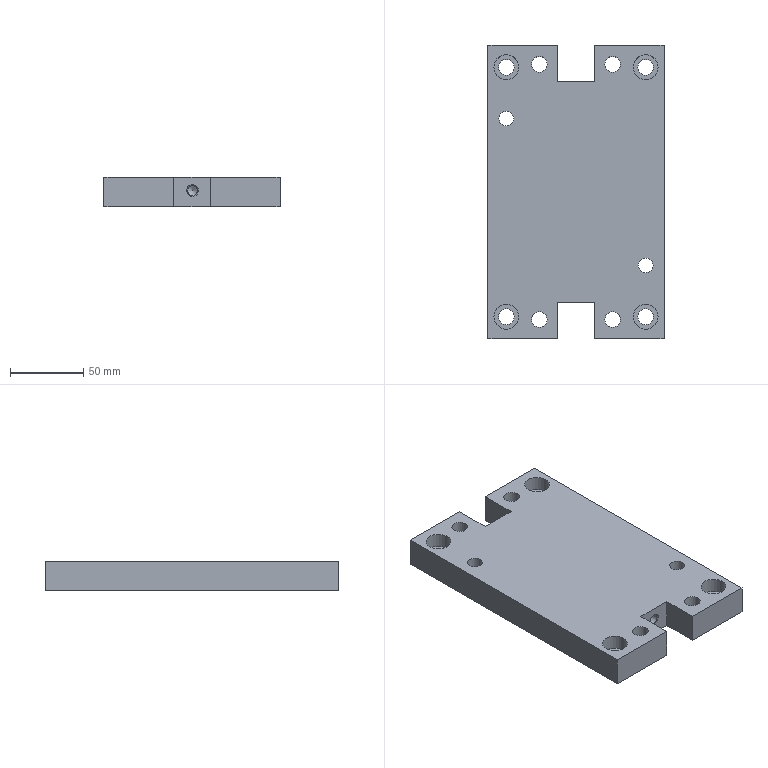Part | STEP file | 冲床-300配套压波_id810_x_t | 1 solid | 46 faces | box 120 x 200 x 20 mm | volume 424966 mm3 | plane 22 | cylinder 20 | cone 4 | commonest cylinder face diameters 10.7 x8 17 x8 6.8 x2 10 x2
STEP:
#1=CARTESIAN_POINT('',(1589.65,87.,10.));
#2=VERTEX_POINT('',#1);
#3=CARTESIAN_POINT('',(1595.,87.,10.));
#4=DIRECTION('',(0.,0.,-1.));
#5=DIRECTION('',(-1.,0.,0.));
#6=AXIS2_PLACEMENT_3D('',#3,#4,#5);
#7=CIRCLE('',#6,5.35);
#8=EDGE_CURVE('',#2,#2,#7,.T.);
#9=ORIENTED_EDGE('',*,*,#8,.F.);
#10=EDGE_LOOP('',(#9));
#11=FACE_BOUND('',#10,.T.);
#12=CARTESIAN_POINT('',(1586.5,87.,10.));
#13=VERTEX_POINT('',#12);
#14=CARTESIAN_POINT('',(1595.,87.,10.));
#15=DIRECTION('',(0.,0.,-1.));
#16=DIRECTION('',(-1.,0.,0.));
#17=AXIS2_PLACEMENT_3D('',#14,#15,#16);
#18=CIRCLE('',#17,8.5);
#19=EDGE_CURVE('',#13,#13,#18,.T.);
#20=ORIENTED_EDGE('',*,*,#19,.T.);
#21=EDGE_LOOP('',(#20));
#22=FACE_BOUND('',#21,.T.);
#23=CARTESIAN_POINT('',(1595.,87.,10.));
#24=DIRECTION('',(0.,0.,1.));
#25=DIRECTION('',(-1.,0.,0.));
#26=AXIS2_PLACEMENT_3D('',#23,#24,#25);
#27=PLANE('',#26);
#28=ADVANCED_FACE('',(#11,#22),#27,.F.);
#29=ORIENTED_EDGE('',*,*,#19,.F.);
#30=EDGE_LOOP('',(#29));
#31=FACE_BOUND('',#30,.T.);
#32=CARTESIAN_POINT('',(1586.5,87.,0.));
#33=VERTEX_POINT('',#32);
#34=CARTESIAN_POINT('',(1595.,87.,0.));
#35=DIRECTION('',(0.,0.,1.));
#36=DIRECTION('',(-1.,0.,0.));
#37=AXIS2_PLACEMENT_3D('',#34,#35,#36);
#38=CIRCLE('',#37,8.5);
#39=EDGE_CURVE('',#33,#33,#38,.T.);
#40=ORIENTED_EDGE('',*,*,#39,.F.);
#41=EDGE_LOOP('',(#40));
#42=FACE_BOUND('',#41,.T.);
#43=CARTESIAN_POINT('',(1595.,87.,0.));
#44=DIRECTION('',(0.,0.,1.));
#45=DIRECTION('',(-1.,0.,0.));
#46=AXIS2_PLACEMENT_3D('',#43,#44,#45);
#47=CYLINDRICAL_SURFACE('',#46,8.5);
#48=ADVANCED_FACE('',(#31,#42),#47,.F.);
#49=CARTESIAN_POINT('',(1589.65,87.,20.));
#50=VERTEX_POINT('',#49);
#51=CARTESIAN_POINT('',(1595.,87.,20.));
#52=DIRECTION('',(0.,0.,-1.));
#53=DIRECTION('',(-1.,0.,0.));
#54=AXIS2_PLACEMENT_3D('',#51,#52,#53);
#55=CIRCLE('',#54,5.35);
#56=EDGE_CURVE('',#50,#50,#55,.T.);
#57=ORIENTED_EDGE('',*,*,#56,.F.);
#58=EDGE_LOOP('',(#57));
#59=FACE_BOUND('',#58,.T.);
#60=ORIENTED_EDGE('',*,*,#8,.T.);
#61=EDGE_LOOP('',(#60));
#62=FACE_BOUND('',#61,.T.);
#63=CARTESIAN_POINT('',(1595.,87.,101.559));
#64=DIRECTION('',(0.,0.,1.));
#65=DIRECTION('',(-1.,0.,0.));
#66=AXIS2_PLACEMENT_3D('',#63,#64,#65);
#67=CYLINDRICAL_SURFACE('',#66,5.35);
#68=ADVANCED_FACE('',(#59,#62),#67,.F.);
#69=CARTESIAN_POINT('',(1623.725,-55.,11.));
#70=VERTEX_POINT('',#69);
#71=CARTESIAN_POINT('',(1620.325,-55.,11.));
#72=DIRECTION('',(0.,-1.,0.));
#73=DIRECTION('',(1.,0.,0.));
#74=AXIS2_PLACEMENT_3D('',#71,#72,#73);
#75=CIRCLE('',#74,3.4);
#76=EDGE_CURVE('',#70,#70,#75,.T.);
#77=ORIENTED_EDGE('',*,*,#76,.T.);
#78=EDGE_LOOP('',(#77));
#79=FACE_BOUND('',#78,.T.);
#80=CARTESIAN_POINT('',(1620.325,-52.957,11.));
#81=VERTEX_POINT('',#80);
#82=VERTEX_LOOP('',#81);
#83=FACE_BOUND('',#82,.T.);
#84=CARTESIAN_POINT('',(1620.325,-55.,11.));
#85=DIRECTION('',(0.,-1.,0.));
#86=DIRECTION('',(-1.,0.,0.));
#87=AXIS2_PLACEMENT_3D('',#84,#85,#86);
#88=CONICAL_SURFACE('',#87,3.4,59.);
#89=ADVANCED_FACE('',(#79,#83),#88,.F.);
#90=CARTESIAN_POINT('',(1623.725,55.,11.));
#91=VERTEX_POINT('',#90);
#92=CARTESIAN_POINT('',(1620.325,55.,11.));
#93=DIRECTION('',(0.,1.,0.));
#94=DIRECTION('',(1.,0.,0.));
#95=AXIS2_PLACEMENT_3D('',#92,#93,#94);
#96=CIRCLE('',#95,3.4);
#97=EDGE_CURVE('',#91,#91,#96,.T.);
#98=ORIENTED_EDGE('',*,*,#97,.T.);
#99=EDGE_LOOP('',(#98));
#100=FACE_BOUND('',#99,.T.);
#101=CARTESIAN_POINT('',(1620.325,52.957,11.));
#102=VERTEX_POINT('',#101);
#103=VERTEX_LOOP('',#102);
#104=FACE_BOUND('',#103,.T.);
#105=CARTESIAN_POINT('',(1620.325,55.,11.));
#106=DIRECTION('',(0.,1.,0.));
#107=DIRECTION('',(-1.,0.,0.));
#108=AXIS2_PLACEMENT_3D('',#105,#106,#107);
#109=CONICAL_SURFACE('',#108,3.4,59.);
#110=ADVANCED_FACE('',(#100,#104),#109,.F.);
#111=CARTESIAN_POINT('',(1620.325,-74.4,14.4));
#112=VERTEX_POINT('',#111);
#113=CARTESIAN_POINT('',(1620.325,-74.4,11.));
#114=DIRECTION('',(0.,-1.,0.));
#115=DIRECTION('',(0.,0.,1.));
#116=AXIS2_PLACEMENT_3D('',#113,#114,#115);
#117=CIRCLE('',#116,3.4);
#118=EDGE_CURVE('',#112,#112,#117,.T.);
#119=ORIENTED_EDGE('',*,*,#118,.T.);
#120=EDGE_LOOP('',(#119));
#121=FACE_BOUND('',#120,.T.);
#122=ORIENTED_EDGE('',*,*,#76,.F.);
#123=EDGE_LOOP('',(#122));
#124=FACE_BOUND('',#123,.T.);
#125=CARTESIAN_POINT('',(1620.325,-75.,11.));
#126=DIRECTION('',(0.,1.,0.));
#127=DIRECTION('',(1.,0.,0.));
#128=AXIS2_PLACEMENT_3D('',#125,#126,#127);
#129=CYLINDRICAL_SURFACE('',#128,3.4);
#130=ADVANCED_FACE('',(#121,#124),#129,.F.);
#131=CARTESIAN_POINT('',(1620.325,74.4,14.4));
#132=VERTEX_POINT('',#131);
#133=CARTESIAN_POINT('',(1620.325,74.4,11.));
#134=DIRECTION('',(0.,1.,0.));
#135=DIRECTION('',(0.,0.,1.));
#136=AXIS2_PLACEMENT_3D('',#133,#134,#135);
#137=CIRCLE('',#136,3.4);
#138=EDGE_CURVE('',#132,#132,#137,.T.);
#139=ORIENTED_EDGE('',*,*,#138,.T.);
#140=EDGE_LOOP('',(#139));
#141=FACE_BOUND('',#140,.T.);
#142=ORIENTED_EDGE('',*,*,#97,.F.);
#143=EDGE_LOOP('',(#142));
#144=FACE_BOUND('',#143,.T.);
#145=CARTESIAN_POINT('',(1620.325,75.,11.));
#146=DIRECTION('',(0.,-1.,0.));
#147=DIRECTION('',(1.,0.,0.));
#148=AXIS2_PLACEMENT_3D('',#145,#146,#147);
#149=CYLINDRICAL_SURFACE('',#148,3.4);
#150=ADVANCED_FACE('',(#141,#144),#149,.F.);
#151=ORIENTED_EDGE('',*,*,#118,.F.);
#152=EDGE_LOOP('',(#151));
#153=FACE_BOUND('',#152,.T.);
#154=CARTESIAN_POINT('',(1616.325,-75.,11.));
#155=VERTEX_POINT('',#154);
#156=CARTESIAN_POINT('',(1620.325,-75.,11.));
#157=DIRECTION('',(0.,1.,0.));
#158=DIRECTION('',(-1.,0.,0.));
#159=AXIS2_PLACEMENT_3D('',#156,#157,#158);
#160=CIRCLE('',#159,4.);
#161=EDGE_CURVE('',#155,#155,#160,.T.);
#162=ORIENTED_EDGE('',*,*,#161,.F.);
#163=EDGE_LOOP('',(#162));
#164=FACE_BOUND('',#163,.T.);
#165=CARTESIAN_POINT('',(1620.325,-75.,11.));
#166=DIRECTION('',(0.,-1.,0.));
#167=DIRECTION('',(0.,0.,1.));
#168=AXIS2_PLACEMENT_3D('',#165,#166,#167);
#169=CONICAL_SURFACE('',#168,4.,45.);
#170=ADVANCED_FACE('',(#153,#164),#169,.F.);
#171=ORIENTED_EDGE('',*,*,#138,.F.);
#172=EDGE_LOOP('',(#171));
#173=FACE_BOUND('',#172,.T.);
#174=CARTESIAN_POINT('',(1616.325,75.,11.));
#175=VERTEX_POINT('',#174);
#176=CARTESIAN_POINT('',(1620.325,75.,11.));
#177=DIRECTION('',(0.,-1.,0.));
#178=DIRECTION('',(-1.,0.,0.));
#179=AXIS2_PLACEMENT_3D('',#176,#177,#178);
#180=CIRCLE('',#179,4.);
#181=EDGE_CURVE('',#175,#175,#180,.T.);
#182=ORIENTED_EDGE('',*,*,#181,.F.);
#183=EDGE_LOOP('',(#182));
#184=FACE_BOUND('',#183,.T.);
#185=CARTESIAN_POINT('',(1620.325,75.,11.));
#186=DIRECTION('',(0.,1.,0.));
#187=DIRECTION('',(0.,0.,1.));
#188=AXIS2_PLACEMENT_3D('',#185,#186,#187);
#189=CONICAL_SURFACE('',#188,4.,45.);
#190=ADVANCED_FACE('',(#173,#184),#189,.F.);
#191=CARTESIAN_POINT('',(1564.,85.,10.));
#192=VERTEX_POINT('',#191);
#193=CARTESIAN_POINT('',(1572.5,85.,10.));
#194=DIRECTION('',(0.,0.,1.));
#195=DIRECTION('',(-1.,0.,0.));
#196=AXIS2_PLACEMENT_3D('',#193,#194,#195);
#197=CIRCLE('',#196,8.5);
#198=EDGE_CURVE('',#192,#192,#197,.T.);
#199=ORIENTED_EDGE('',*,*,#198,.T.);
#200=EDGE_LOOP('',(#199));
#201=FACE_BOUND('',#200,.T.);
#202=CARTESIAN_POINT('',(1567.15,85.,10.));
#203=VERTEX_POINT('',#202);
#204=CARTESIAN_POINT('',(1572.5,85.,10.));
#205=DIRECTION('',(0.,0.,1.));
#206=DIRECTION('',(-1.,0.,0.));
#207=AXIS2_PLACEMENT_3D('',#204,#205,#206);
#208=CIRCLE('',#207,5.35);
#209=EDGE_CURVE('',#203,#203,#208,.T.);
#210=ORIENTED_EDGE('',*,*,#209,.F.);
#211=EDGE_LOOP('',(#210));
#212=FACE_BOUND('',#211,.T.);
#213=CARTESIAN_POINT('',(1572.5,85.,10.));
#214=DIRECTION('',(0.,0.,-1.));
#215=DIRECTION('',(-1.,0.,0.));
#216=AXIS2_PLACEMENT_3D('',#213,#214,#215);
#217=PLANE('',#216);
#218=ADVANCED_FACE('',(#201,#212),#217,.F.);
#219=CARTESIAN_POINT('',(1676.,85.,10.));
#220=VERTEX_POINT('',#219);
#221=CARTESIAN_POINT('',(1667.5,85.,10.));
#222=DIRECTION('',(0.,0.,1.));
#223=DIRECTION('',(1.,0.,0.));
#224=AXIS2_PLACEMENT_3D('',#221,#222,#223);
#225=CIRCLE('',#224,8.5);
#226=EDGE_CURVE('',#220,#220,#225,.T.);
#227=ORIENTED_EDGE('',*,*,#226,.T.);
#228=EDGE_LOOP('',(#227));
#229=FACE_BOUND('',#228,.T.);
#230=CARTESIAN_POINT('',(1672.85,85.,10.));
#231=VERTEX_POINT('',#230);
#232=CARTESIAN_POINT('',(1667.5,85.,10.));
#233=DIRECTION('',(0.,0.,1.));
#234=DIRECTION('',(1.,0.,0.));
#235=AXIS2_PLACEMENT_3D('',#232,#233,#234);
#236=CIRCLE('',#235,5.35);
#237=EDGE_CURVE('',#231,#231,#236,.T.);
#238=ORIENTED_EDGE('',*,*,#237,.F.);
#239=EDGE_LOOP('',(#238));
#240=FACE_BOUND('',#239,.T.);
#241=CARTESIAN_POINT('',(1667.5,85.,10.));
#242=DIRECTION('',(0.,0.,-1.));
#243=DIRECTION('',(1.,0.,0.));
#244=AXIS2_PLACEMENT_3D('',#241,#242,#243);
#245=PLANE('',#244);
#246=ADVANCED_FACE('',(#229,#240),#245,.F.);
#247=CARTESIAN_POINT('',(1564.,-85.,10.));
#248=VERTEX_POINT('',#247);
#249=CARTESIAN_POINT('',(1572.5,-85.,10.));
#250=DIRECTION('',(0.,0.,1.));
#251=DIRECTION('',(-1.,0.,0.));
#252=AXIS2_PLACEMENT_3D('',#249,#250,#251);
#253=CIRCLE('',#252,8.5);
#254=EDGE_CURVE('',#248,#248,#253,.T.);
#255=ORIENTED_EDGE('',*,*,#254,.T.);
#256=EDGE_LOOP('',(#255));
#257=FACE_BOUND('',#256,.T.);
#258=CARTESIAN_POINT('',(1567.15,-85.,10.));
#259=VERTEX_POINT('',#258);
#260=CARTESIAN_POINT('',(1572.5,-85.,10.));
#261=DIRECTION('',(0.,0.,1.));
#262=DIRECTION('',(-1.,0.,0.));
#263=AXIS2_PLACEMENT_3D('',#260,#261,#262);
#264=CIRCLE('',#263,5.35);
#265=EDGE_CURVE('',#259,#259,#264,.T.);
#266=ORIENTED_EDGE('',*,*,#265,.F.);
#267=EDGE_LOOP('',(#266));
#268=FACE_BOUND('',#267,.T.);
#269=CARTESIAN_POINT('',(1572.5,-85.,10.));
#270=DIRECTION('',(0.,0.,-1.));
#271=DIRECTION('',(-1.,0.,0.));
#272=AXIS2_PLACEMENT_3D('',#269,#270,#271);
#273=PLANE('',#272);
#274=ADVANCED_FACE('',(#257,#268),#273,.F.);
#275=CARTESIAN_POINT('',(1676.,-85.,10.));
#276=VERTEX_POINT('',#275);
#277=CARTESIAN_POINT('',(1667.5,-85.,10.));
#278=DIRECTION('',(0.,0.,1.));
#279=DIRECTION('',(1.,0.,0.));
#280=AXIS2_PLACEMENT_3D('',#277,#278,#279);
#281=CIRCLE('',#280,8.5);
#282=EDGE_CURVE('',#276,#276,#281,.T.);
#283=ORIENTED_EDGE('',*,*,#282,.T.);
#284=EDGE_LOOP('',(#283));
#285=FACE_BOUND('',#284,.T.);
#286=CARTESIAN_POINT('',(1672.85,-85.,10.));
#287=VERTEX_POINT('',#286);
#288=CARTESIAN_POINT('',(1667.5,-85.,10.));
#289=DIRECTION('',(0.,0.,1.));
#290=DIRECTION('',(1.,0.,0.));
#291=AXIS2_PLACEMENT_3D('',#288,#289,#290);
#292=CIRCLE('',#291,5.35);
#293=EDGE_CURVE('',#287,#287,#292,.T.);
#294=ORIENTED_EDGE('',*,*,#293,.F.);
#295=EDGE_LOOP('',(#294));
#296=FACE_BOUND('',#295,.T.);
#297=CARTESIAN_POINT('',(1667.5,-85.,10.));
#298=DIRECTION('',(0.,0.,-1.));
#299=DIRECTION('',(1.,0.,0.));
#300=AXIS2_PLACEMENT_3D('',#297,#298,#299);
#301=PLANE('',#300);
#302=ADVANCED_FACE('',(#285,#296),#301,.F.);
#303=CARTESIAN_POINT('',(1650.35,-87.,10.));
#304=VERTEX_POINT('',#303);
#305=CARTESIAN_POINT('',(1645.,-87.,10.));
#306=DIRECTION('',(0.,0.,-1.));
#307=DIRECTION('',(1.,0.,0.));
#308=AXIS2_PLACEMENT_3D('',#305,#306,#307);
#309=CIRCLE('',#308,5.35);
#310=EDGE_CURVE('',#304,#304,#309,.T.);
#311=ORIENTED_EDGE('',*,*,#310,.F.);
#312=EDGE_LOOP('',(#311));
#313=FACE_BOUND('',#312,.T.);
#314=CARTESIAN_POINT('',(1653.5,-87.,10.));
#315=VERTEX_POINT('',#314);
#316=CARTESIAN_POINT('',(1645.,-87.,10.));
#317=DIRECTION('',(0.,0.,-1.));
#318=DIRECTION('',(1.,0.,0.));
#319=AXIS2_PLACEMENT_3D('',#316,#317,#318);
#320=CIRCLE('',#319,8.5);
#321=EDGE_CURVE('',#315,#315,#320,.T.);
#322=ORIENTED_EDGE('',*,*,#321,.T.);
#323=EDGE_LOOP('',(#322));
#324=FACE_BOUND('',#323,.T.);
#325=CARTESIAN_POINT('',(1645.,-87.,10.));
#326=DIRECTION('',(0.,0.,1.));
#327=DIRECTION('',(1.,0.,0.));
#328=AXIS2_PLACEMENT_3D('',#325,#326,#327);
#329=PLANE('',#328);
#330=ADVANCED_FACE('',(#313,#324),#329,.F.);
#331=CARTESIAN_POINT('',(1589.65,-87.,10.));
#332=VERTEX_POINT('',#331);
#333=CARTESIAN_POINT('',(1595.,-87.,10.));
#334=DIRECTION('',(0.,0.,-1.));
#335=DIRECTION('',(-1.,0.,0.));
#336=AXIS2_PLACEMENT_3D('',#333,#334,#335);
#337=CIRCLE('',#336,5.35);
#338=EDGE_CURVE('',#332,#332,#337,.T.);
#339=ORIENTED_EDGE('',*,*,#338,.F.);
#340=EDGE_LOOP('',(#339));
#341=FACE_BOUND('',#340,.T.);
#342=CARTESIAN_POINT('',(1586.5,-87.,10.));
#343=VERTEX_POINT('',#342);
#344=CARTESIAN_POINT('',(1595.,-87.,10.));
#345=DIRECTION('',(0.,0.,-1.));
#346=DIRECTION('',(-1.,0.,0.));
#347=AXIS2_PLACEMENT_3D('',#344,#345,#346);
#348=CIRCLE('',#347,8.5);
#349=EDGE_CURVE('',#343,#343,#348,.T.);
#350=ORIENTED_EDGE('',*,*,#349,.T.);
#351=EDGE_LOOP('',(#350));
#352=FACE_BOUND('',#351,.T.);
#353=CARTESIAN_POINT('',(1595.,-87.,10.));
#354=DIRECTION('',(0.,0.,1.));
#355=DIRECTION('',(-1.,0.,0.));
#356=AXIS2_PLACEMENT_3D('',#353,#354,#355);
#357=PLANE('',#356);
#358=ADVANCED_FACE('',(#341,#352),#357,.F.);
#359=CARTESIAN_POINT('',(1564.,85.,20.));
#360=VERTEX_POINT('',#359);
#361=CARTESIAN_POINT('',(1572.5,85.,20.));
#362=DIRECTION('',(0.,0.,-1.));
#363=DIRECTION('',(-1.,0.,0.));
#364=AXIS2_PLACEMENT_3D('',#361,#362,#363);
#365=CIRCLE('',#364,8.5);
#366=EDGE_CURVE('',#360,#360,#365,.T.);
#367=ORIENTED_EDGE('',*,*,#366,.F.);
#368=EDGE_LOOP('',(#367));
#369=FACE_BOUND('',#368,.T.);
#370=ORIENTED_EDGE('',*,*,#198,.F.);
#371=EDGE_LOOP('',(#370));
#372=FACE_BOUND('',#371,.T.);
#373=CARTESIAN_POINT('',(1572.5,85.,20.));
#374=DIRECTION('',(0.,0.,-1.));
#375=DIRECTION('',(-1.,0.,0.));
#376=AXIS2_PLACEMENT_3D('',#373,#374,#375);
#377=CYLINDRICAL_SURFACE('',#376,8.5);
#378=ADVANCED_FACE('',(#369,#372),#377,.F.);
#379=CARTESIAN_POINT('',(1672.5,-50.,20.));
#380=VERTEX_POINT('',#379);
#381=CARTESIAN_POINT('',(1667.5,-50.,20.));
#382=DIRECTION('',(0.,0.,-1.));
#383=DIRECTION('',(1.,0.,0.));
#384=AXIS2_PLACEMENT_3D('',#381,#382,#383);
#385=CIRCLE('',#384,5.);
#386=EDGE_CURVE('',#380,#380,#385,.T.);
#387=ORIENTED_EDGE('',*,*,#386,.F.);
#388=EDGE_LOOP('',(#387));
#389=FACE_BOUND('',#388,.T.);
#390=CARTESIAN_POINT('',(1672.5,-50.,0.));
#391=VERTEX_POINT('',#390);
#392=CARTESIAN_POINT('',(1667.5,-50.,0.));
#393=DIRECTION('',(0.,0.,-1.));
#394=DIRECTION('',(1.,0.,0.));
#395=AXIS2_PLACEMENT_3D('',#392,#393,#394);
#396=CIRCLE('',#395,5.);
#397=EDGE_CURVE('',#391,#391,#396,.T.);
#398=ORIENTED_EDGE('',*,*,#397,.T.);
#399=EDGE_LOOP('',(#398));
#400=FACE_BOUND('',#399,.T.);
#401=CARTESIAN_POINT('',(1667.5,-50.,129.));
#402=DIRECTION('',(0.,0.,-1.));
#403=DIRECTION('',(-1.,0.,0.));
#404=AXIS2_PLACEMENT_3D('',#401,#402,#403);
#405=CYLINDRICAL_SURFACE('',#404,5.);
#406=ADVANCED_FACE('',(#389,#400),#405,.F.);
#407=ORIENTED_EDGE('',*,*,#161,.T.);
#408=EDGE_LOOP('',(#407));
#409=FACE_BOUND('',#408,.T.);
#410=CARTESIAN_POINT('',(1607.485,-75.,0.));
#411=VERTEX_POINT('',#410);
#412=CARTESIAN_POINT('',(1607.485,-75.,20.));
#413=VERTEX_POINT('',#412);
#414=CARTESIAN_POINT('',(1607.485,-75.,-18.315));
#415=DIRECTION('',(0.,0.,1.));
#416=VECTOR('',#415,1.);
#417=LINE('',#414,#416);
#418=EDGE_CURVE('',#411,#413,#417,.T.);
#419=ORIENTED_EDGE('',*,*,#418,.F.);
#420=CARTESIAN_POINT('',(1632.515,-75.,0.));
#421=VERTEX_POINT('',#420);
#422=CARTESIAN_POINT('',(1660.,-75.,0.));
#423=DIRECTION('',(-1.,0.,0.));
#424=VECTOR('',#423,1.);
#425=LINE('',#422,#424);
#426=EDGE_CURVE('',#421,#411,#425,.T.);
#427=ORIENTED_EDGE('',*,*,#426,.F.);
#428=CARTESIAN_POINT('',(1632.515,-75.,20.));
#429=VERTEX_POINT('',#428);
#430=CARTESIAN_POINT('',(1632.515,-75.,37.685));
#431=DIRECTION('',(0.,0.,-1.));
#432=VECTOR('',#431,1.);
#433=LINE('',#430,#432);
#434=EDGE_CURVE('',#429,#421,#433,.T.);
#435=ORIENTED_EDGE('',*,*,#434,.F.);
#436=CARTESIAN_POINT('',(1660.,-75.,20.));
#437=DIRECTION('',(1.,0.,0.));
#438=VECTOR('',#437,1.);
#439=LINE('',#436,#438);
#440=EDGE_CURVE('',#413,#429,#439,.T.);
#441=ORIENTED_EDGE('',*,*,#440,.F.);
#442=EDGE_LOOP('',(#419,#427,#435,#441));
#443=FACE_BOUND('',#442,.T.);
#444=CARTESIAN_POINT('',(1560.,-75.,170.));
#445=DIRECTION('',(0.,-1.,0.));
#446=DIRECTION('',(-1.,0.,0.));
#447=AXIS2_PLACEMENT_3D('',#444,#445,#446);
#448=PLANE('',#447);
#449=ADVANCED_FACE('',(#409,#443),#448,.T.);
#450=CARTESIAN_POINT('',(1632.515,-100.,20.));
#451=VERTEX_POINT('',#450);
#452=CARTESIAN_POINT('',(1632.515,0.,20.));
#453=DIRECTION('',(0.,1.,0.));
#454=VECTOR('',#453,1.);
#455=LINE('',#452,#454);
#456=EDGE_CURVE('',#451,#429,#455,.T.);
#457=ORIENTED_EDGE('',*,*,#456,.T.);
#458=ORIENTED_EDGE('',*,*,#434,.T.);
#459=CARTESIAN_POINT('',(1632.515,-100.,0.));
#460=VERTEX_POINT('',#459);
#461=CARTESIAN_POINT('',(1632.515,-75.,0.));
#462=DIRECTION('',(0.,-1.,0.));
#463=VECTOR('',#462,1.);
#464=LINE('',#461,#463);
#465=EDGE_CURVE('',#421,#460,#464,.T.);
#466=ORIENTED_EDGE('',*,*,#465,.T.);
#467=CARTESIAN_POINT('',(1632.515,-100.,37.685));
#468=DIRECTION('',(0.,0.,1.));
#469=VECTOR('',#468,1.);
#470=LINE('',#467,#469);
#471=EDGE_CURVE('',#460,#451,#470,.T.);
#472=ORIENTED_EDGE('',*,*,#471,.T.);
#473=EDGE_LOOP('',(#457,#458,#466,#472));
#474=FACE_OUTER_BOUND('',#473,.T.);
#475=CARTESIAN_POINT('',(1632.515,-75.,37.685));
#476=DIRECTION('',(1.,0.,0.));
#477=DIRECTION('',(0.,0.,-1.));
#478=AXIS2_PLACEMENT_3D('',#475,#476,#477);
#479=PLANE('',#478);
#480=ADVANCED_FACE('',(#474),#479,.F.);
#481=ORIENTED_EDGE('',*,*,#471,.F.);
#482=CARTESIAN_POINT('',(1680.,-100.,0.));
#483=VERTEX_POINT('',#482);
#484=CARTESIAN_POINT('',(1560.,-100.,0.));
#485=DIRECTION('',(1.,0.,0.));
#486=VECTOR('',#485,1.);
#487=LINE('',#484,#486);
#488=EDGE_CURVE('',#460,#483,#487,.T.);
#489=ORIENTED_EDGE('',*,*,#488,.T.);
#490=CARTESIAN_POINT('',(1680.,-100.,20.));
#491=VERTEX_POINT('',#490);
#492=CARTESIAN_POINT('',(1680.,-100.,170.));
#493=DIRECTION('',(0.,0.,-1.));
#494=VECTOR('',#493,1.);
#495=LINE('',#492,#494);
#496=EDGE_CURVE('',#491,#483,#495,.T.);
#497=ORIENTED_EDGE('',*,*,#496,.F.);
#498=CARTESIAN_POINT('',(1560.,-100.,20.));
#499=DIRECTION('',(1.,0.,0.));
#500=VECTOR('',#499,1.);
#501=LINE('',#498,#500);
#502=EDGE_CURVE('',#451,#491,#501,.T.);
#503=ORIENTED_EDGE('',*,*,#502,.F.);
#504=EDGE_LOOP('',(#481,#489,#497,#503));
#505=FACE_OUTER_BOUND('',#504,.T.);
#506=CARTESIAN_POINT('',(1560.,-100.,20.));
#507=DIRECTION('',(0.,1.,0.));
#508=DIRECTION('',(-1.,0.,0.));
#509=AXIS2_PLACEMENT_3D('',#506,#507,#508);
#510=PLANE('',#509);
#511=ADVANCED_FACE('',(#505),#510,.F.);
#512=CARTESIAN_POINT('',(1680.,100.,0.));
#513=VERTEX_POINT('',#512);
#514=CARTESIAN_POINT('',(1680.,75.,0.));
#515=DIRECTION('',(0.,1.,0.));
#516=VECTOR('',#515,1.);
#517=LINE('',#514,#516);
#518=EDGE_CURVE('',#483,#513,#517,.T.);
#519=ORIENTED_EDGE('',*,*,#518,.T.);
#520=CARTESIAN_POINT('',(1680.,100.,20.));
#521=VERTEX_POINT('',#520);
#522=CARTESIAN_POINT('',(1680.,100.,20.));
#523=DIRECTION('',(0.,0.,-1.));
#524=VECTOR('',#523,1.);
#525=LINE('',#522,#524);
#526=EDGE_CURVE('',#521,#513,#525,.T.);
#527=ORIENTED_EDGE('',*,*,#526,.F.);
#528=CARTESIAN_POINT('',(1680.,75.,20.));
#529=DIRECTION('',(0.,1.,0.));
#530=VECTOR('',#529,1.);
#531=LINE('',#528,#530);
#532=EDGE_CURVE('',#491,#521,#531,.T.);
#533=ORIENTED_EDGE('',*,*,#532,.F.);
#534=ORIENTED_EDGE('',*,*,#496,.T.);
#535=EDGE_LOOP('',(#519,#527,#533,#534));
#536=FACE_OUTER_BOUND('',#535,.T.);
#537=CARTESIAN_POINT('',(1680.,75.,170.));
#538=DIRECTION('',(-1.,0.,0.));
#539=DIRECTION('',(0.,0.,1.));
#540=AXIS2_PLACEMENT_3D('',#537,#538,#539);
#541=PLANE('',#540);
#542=ADVANCED_FACE('',(#536),#541,.F.);
#543=CARTESIAN_POINT('',(1632.515,100.,20.));
#544=VERTEX_POINT('',#543);
#545=CARTESIAN_POINT('',(1632.515,100.,0.));
#546=VERTEX_POINT('',#545);
#547=CARTESIAN_POINT('',(1632.515,100.,37.685));
#548=DIRECTION('',(0.,0.,-1.));
#549=VECTOR('',#548,1.);
#550=LINE('',#547,#549);
#551=EDGE_CURVE('',#544,#546,#550,.T.);
#552=ORIENTED_EDGE('',*,*,#551,.F.);
#553=CARTESIAN_POINT('',(1680.,100.,20.));
#554=DIRECTION('',(-1.,0.,0.));
#555=VECTOR('',#554,1.);
#556=LINE('',#553,#555);
#557=EDGE_CURVE('',#521,#544,#556,.T.);
#558=ORIENTED_EDGE('',*,*,#557,.F.);
#559=ORIENTED_EDGE('',*,*,#526,.T.);
#560=CARTESIAN_POINT('',(1680.,100.,0.));
#561=DIRECTION('',(-1.,0.,0.));
#562=VECTOR('',#561,1.);
#563=LINE('',#560,#562);
#564=EDGE_CURVE('',#513,#546,#563,.T.);
#565=ORIENTED_EDGE('',*,*,#564,.T.);
#566=EDGE_LOOP('',(#552,#558,#559,#565));
#567=FACE_OUTER_BOUND('',#566,.T.);
#568=CARTESIAN_POINT('',(1680.,100.,20.));
#569=DIRECTION('',(0.,-1.,0.));
#570=DIRECTION('',(1.,0.,0.));
#571=AXIS2_PLACEMENT_3D('',#568,#569,#570);
#572=PLANE('',#571);
#573=ADVANCED_FACE('',(#567),#572,.F.);
#574=CARTESIAN_POINT('',(1632.515,75.,0.));
#575=VERTEX_POINT('',#574);
#576=CARTESIAN_POINT('',(1632.515,75.,20.));
#577=VERTEX_POINT('',#576);
#578=CARTESIAN_POINT('',(1632.515,75.,37.685));
#579=DIRECTION('',(0.,0.,1.));
#580=VECTOR('',#579,1.);
#581=LINE('',#578,#580);
#582=EDGE_CURVE('',#575,#577,#581,.T.);
#583=ORIENTED_EDGE('',*,*,#582,.T.);
#584=CARTESIAN_POINT('',(1632.515,0.,20.));
#585=DIRECTION('',(0.,1.,0.));
#586=VECTOR('',#585,1.);
#587=LINE('',#584,#586);
#588=EDGE_CURVE('',#577,#544,#587,.T.);
#589=ORIENTED_EDGE('',*,*,#588,.T.);
#590=ORIENTED_EDGE('',*,*,#551,.T.);
#591=CARTESIAN_POINT('',(1632.515,0.,0.));
#592=DIRECTION('',(0.,1.,0.));
#593=VECTOR('',#592,1.);
#594=LINE('',#591,#593);
#595=EDGE_CURVE('',#575,#546,#594,.T.);
#596=ORIENTED_EDGE('',*,*,#595,.F.);
#597=EDGE_LOOP('',(#583,#589,#590,#596));
#598=FACE_OUTER_BOUND('',#597,.T.);
#599=CARTESIAN_POINT('',(1632.515,75.,37.685));
#600=DIRECTION('',(1.,0.,0.));
#601=DIRECTION('',(0.,0.,-1.));
#602=AXIS2_PLACEMENT_3D('',#599,#600,#601);
#603=PLANE('',#602);
#604=ADVANCED_FACE('',(#598),#603,.F.);
#605=ORIENTED_EDGE('',*,*,#181,.T.);
#606=EDGE_LOOP('',(#605));
#607=FACE_BOUND('',#606,.T.);
#608=ORIENTED_EDGE('',*,*,#582,.F.);
#609=CARTESIAN_POINT('',(1607.485,75.,0.));
#610=VERTEX_POINT('',#609);
#611=CARTESIAN_POINT('',(1660.,75.,0.));
#612=DIRECTION('',(-1.,0.,0.));
#613=VECTOR('',#612,1.);
#614=LINE('',#611,#613);
#615=EDGE_CURVE('',#575,#610,#614,.T.);
#616=ORIENTED_EDGE('',*,*,#615,.T.);
#617=CARTESIAN_POINT('',(1607.485,75.,20.));
#618=VERTEX_POINT('',#617);
#619=CARTESIAN_POINT('',(1607.485,75.,-18.315));
#620=DIRECTION('',(0.,0.,-1.));
#621=VECTOR('',#620,1.);
#622=LINE('',#619,#621);
#623=EDGE_CURVE('',#618,#610,#622,.T.);
#624=ORIENTED_EDGE('',*,*,#623,.F.);
#625=CARTESIAN_POINT('',(1660.,75.,20.));
#626=DIRECTION('',(-1.,0.,0.));
#627=VECTOR('',#626,1.);
#628=LINE('',#625,#627);
#629=EDGE_CURVE('',#577,#618,#628,.T.);
#630=ORIENTED_EDGE('',*,*,#629,.F.);
#631=EDGE_LOOP('',(#608,#616,#624,#630));
#632=FACE_BOUND('',#631,.T.);
#633=CARTESIAN_POINT('',(1560.,75.,170.));
#634=DIRECTION('',(0.,1.,0.));
#635=DIRECTION('',(-1.,0.,0.));
#636=AXIS2_PLACEMENT_3D('',#633,#634,#635);
#637=PLANE('',#636);
#638=ADVANCED_FACE('',(#607,#632),#637,.T.);
#639=CARTESIAN_POINT('',(1607.485,100.,0.));
#640=VERTEX_POINT('',#639);
#641=CARTESIAN_POINT('',(1607.485,100.,20.));
#642=VERTEX_POINT('',#641);
#643=CARTESIAN_POINT('',(1607.485,100.,-18.315));
#644=DIRECTION('',(0.,0.,1.));
#645=VECTOR('',#644,1.);
#646=LINE('',#643,#645);
#647=EDGE_CURVE('',#640,#642,#646,.T.);
#648=ORIENTED_EDGE('',*,*,#647,.T.);
#649=CARTESIAN_POINT('',(1607.485,0.,20.));
#650=DIRECTION('',(0.,-1.,0.));
#651=VECTOR('',#650,1.);
#652=LINE('',#649,#651);
#653=EDGE_CURVE('',#642,#618,#652,.T.);
#654=ORIENTED_EDGE('',*,*,#653,.T.);
#655=ORIENTED_EDGE('',*,*,#623,.T.);
#656=CARTESIAN_POINT('',(1607.485,0.,0.));
#657=DIRECTION('',(0.,-1.,0.));
#658=VECTOR('',#657,1.);
#659=LINE('',#656,#658);
#660=EDGE_CURVE('',#640,#610,#659,.T.);
#661=ORIENTED_EDGE('',*,*,#660,.F.);
#662=EDGE_LOOP('',(#648,#654,#655,#661));
#663=FACE_OUTER_BOUND('',#662,.T.);
#664=CARTESIAN_POINT('',(1607.485,75.,-18.315));
#665=DIRECTION('',(-1.,0.,0.));
#666=DIRECTION('',(0.,0.,1.));
#667=AXIS2_PLACEMENT_3D('',#664,#665,#666);
#668=PLANE('',#667);
#669=ADVANCED_FACE('',(#663),#668,.F.);
#670=ORIENTED_EDGE('',*,*,#647,.F.);
#671=CARTESIAN_POINT('',(1560.,100.,0.));
#672=VERTEX_POINT('',#671);
#673=CARTESIAN_POINT('',(1680.,100.,0.));
#674=DIRECTION('',(-1.,0.,0.));
#675=VECTOR('',#674,1.);
#676=LINE('',#673,#675);
#677=EDGE_CURVE('',#640,#672,#676,.T.);
#678=ORIENTED_EDGE('',*,*,#677,.T.);
#679=CARTESIAN_POINT('',(1560.,100.,20.));
#680=VERTEX_POINT('',#679);
#681=CARTESIAN_POINT('',(1560.,100.,170.));
#682=DIRECTION('',(0.,0.,-1.));
#683=VECTOR('',#682,1.);
#684=LINE('',#681,#683);
#685=EDGE_CURVE('',#680,#672,#684,.T.);
#686=ORIENTED_EDGE('',*,*,#685,.F.);
#687=CARTESIAN_POINT('',(1680.,100.,20.));
#688=DIRECTION('',(-1.,0.,0.));
#689=VECTOR('',#688,1.);
#690=LINE('',#687,#689);
#691=EDGE_CURVE('',#642,#680,#690,.T.);
#692=ORIENTED_EDGE('',*,*,#691,.F.);
#693=EDGE_LOOP('',(#670,#678,#686,#692));
#694=FACE_OUTER_BOUND('',#693,.T.);
#695=CARTESIAN_POINT('',(1680.,100.,20.));
#696=DIRECTION('',(0.,-1.,0.));
#697=DIRECTION('',(1.,0.,0.));
#698=AXIS2_PLACEMENT_3D('',#695,#696,#697);
#699=PLANE('',#698);
#700=ADVANCED_FACE('',(#694),#699,.F.);
#701=CARTESIAN_POINT('',(1560.,-100.,0.));
#702=VERTEX_POINT('',#701);
#703=CARTESIAN_POINT('',(1560.,-100.,0.));
#704=DIRECTION('',(0.,-1.,0.));
#705=VECTOR('',#704,1.);
#706=LINE('',#703,#705);
#707=EDGE_CURVE('',#672,#702,#706,.T.);
#708=ORIENTED_EDGE('',*,*,#707,.T.);
#709=CARTESIAN_POINT('',(1560.,-100.,20.));
#710=VERTEX_POINT('',#709);
#711=CARTESIAN_POINT('',(1560.,-100.,20.));
#712=DIRECTION('',(0.,0.,-1.));
#713=VECTOR('',#712,1.);
#714=LINE('',#711,#713);
#715=EDGE_CURVE('',#710,#702,#714,.T.);
#716=ORIENTED_EDGE('',*,*,#715,.F.);
#717=CARTESIAN_POINT('',(1560.,-100.,20.));
#718=DIRECTION('',(0.,-1.,0.));
#719=VECTOR('',#718,1.);
#720=LINE('',#717,#719);
#721=EDGE_CURVE('',#680,#710,#720,.T.);
#722=ORIENTED_EDGE('',*,*,#721,.F.);
#723=ORIENTED_EDGE('',*,*,#685,.T.);
#724=EDGE_LOOP('',(#708,#716,#722,#723));
#725=FACE_OUTER_BOUND('',#724,.T.);
#726=CARTESIAN_POINT('',(1560.,-100.,170.));
#727=DIRECTION('',(1.,0.,0.));
#728=DIRECTION('',(0.,0.,-1.));
#729=AXIS2_PLACEMENT_3D('',#726,#727,#728);
#730=PLANE('',#729);
#731=ADVANCED_FACE('',(#725),#730,.F.);
#732=CARTESIAN_POINT('',(1607.485,-100.,20.));
#733=VERTEX_POINT('',#732);
#734=CARTESIAN_POINT('',(1607.485,-100.,0.));
#735=VERTEX_POINT('',#734);
#736=CARTESIAN_POINT('',(1607.485,-100.,-18.315));
#737=DIRECTION('',(0.,0.,-1.));
#738=VECTOR('',#737,1.);
#739=LINE('',#736,#738);
#740=EDGE_CURVE('',#733,#735,#739,.T.);
#741=ORIENTED_EDGE('',*,*,#740,.F.);
#742=CARTESIAN_POINT('',(1560.,-100.,20.));
#743=DIRECTION('',(1.,0.,0.));
#744=VECTOR('',#743,1.);
#745=LINE('',#742,#744);
#746=EDGE_CURVE('',#710,#733,#745,.T.);
#747=ORIENTED_EDGE('',*,*,#746,.F.);
#748=ORIENTED_EDGE('',*,*,#715,.T.);
#749=CARTESIAN_POINT('',(1560.,-100.,0.));
#750=DIRECTION('',(1.,0.,0.));
#751=VECTOR('',#750,1.);
#752=LINE('',#749,#751);
#753=EDGE_CURVE('',#702,#735,#752,.T.);
#754=ORIENTED_EDGE('',*,*,#753,.T.);
#755=EDGE_LOOP('',(#741,#747,#748,#754));
#756=FACE_OUTER_BOUND('',#755,.T.);
#757=CARTESIAN_POINT('',(1560.,-100.,20.));
#758=DIRECTION('',(0.,1.,0.));
#759=DIRECTION('',(-1.,0.,0.));
#760=AXIS2_PLACEMENT_3D('',#757,#758,#759);
#761=PLANE('',#760);
#762=ADVANCED_FACE('',(#756),#761,.F.);
#763=CARTESIAN_POINT('',(1607.485,0.,20.));
#764=DIRECTION('',(0.,-1.,0.));
#765=VECTOR('',#764,1.);
#766=LINE('',#763,#765);
#767=EDGE_CURVE('',#413,#733,#766,.T.);
#768=ORIENTED_EDGE('',*,*,#767,.T.);
#769=ORIENTED_EDGE('',*,*,#740,.T.);
#770=CARTESIAN_POINT('',(1607.485,0.,0.));
#771=DIRECTION('',(0.,-1.,0.));
#772=VECTOR('',#771,1.);
#773=LINE('',#770,#772);
#774=EDGE_CURVE('',#411,#735,#773,.T.);
#775=ORIENTED_EDGE('',*,*,#774,.F.);
#776=ORIENTED_EDGE('',*,*,#418,.T.);
#777=EDGE_LOOP('',(#768,#769,#775,#776));
#778=FACE_OUTER_BOUND('',#777,.T.);
#779=CARTESIAN_POINT('',(1607.485,-75.,-18.315));
#780=DIRECTION('',(-1.,0.,0.));
#781=DIRECTION('',(0.,0.,1.));
#782=AXIS2_PLACEMENT_3D('',#779,#780,#781);
#783=PLANE('',#782);
#784=ADVANCED_FACE('',(#778),#783,.F.);
#785=ORIENTED_EDGE('',*,*,#209,.T.);
#786=EDGE_LOOP('',(#785));
#787=FACE_BOUND('',#786,.T.);
#788=CARTESIAN_POINT('',(1577.85,85.,0.));
#789=VERTEX_POINT('',#788);
#790=CARTESIAN_POINT('',(1572.5,85.,0.));
#791=DIRECTION('',(0.,0.,1.));
#792=DIRECTION('',(1.,0.,0.));
#793=AXIS2_PLACEMENT_3D('',#790,#791,#792);
#794=CIRCLE('',#793,5.35);
#795=EDGE_CURVE('',#789,#789,#794,.T.);
#796=ORIENTED_EDGE('',*,*,#795,.F.);
#797=EDGE_LOOP('',(#796));
#798=FACE_BOUND('',#797,.T.);
#799=CARTESIAN_POINT('',(1572.5,85.,-74.236));
#800=DIRECTION('',(0.,0.,-1.));
#801=DIRECTION('',(-1.,0.,0.));
#802=AXIS2_PLACEMENT_3D('',#799,#800,#801);
#803=CYLINDRICAL_SURFACE('',#802,5.35);
#804=ADVANCED_FACE('',(#787,#798),#803,.F.);
#805=CARTESIAN_POINT('',(1577.5,50.,20.));
#806=VERTEX_POINT('',#805);
#807=CARTESIAN_POINT('',(1572.5,50.,20.));
#808=DIRECTION('',(0.,0.,1.));
#809=DIRECTION('',(1.,0.,0.));
#810=AXIS2_PLACEMENT_3D('',#807,#808,#809);
#811=CIRCLE('',#810,5.);
#812=EDGE_CURVE('',#806,#806,#811,.T.);
#813=ORIENTED_EDGE('',*,*,#812,.T.);
#814=EDGE_LOOP('',(#813));
#815=FACE_BOUND('',#814,.T.);
#816=CARTESIAN_POINT('',(1577.5,50.,0.));
#817=VERTEX_POINT('',#816);
#818=CARTESIAN_POINT('',(1572.5,50.,0.));
#819=DIRECTION('',(0.,0.,1.));
#820=DIRECTION('',(1.,0.,0.));
#821=AXIS2_PLACEMENT_3D('',#818,#819,#820);
#822=CIRCLE('',#821,5.);
#823=EDGE_CURVE('',#817,#817,#822,.T.);
#824=ORIENTED_EDGE('',*,*,#823,.F.);
#825=EDGE_LOOP('',(#824));
#826=FACE_BOUND('',#825,.T.);
#827=CARTESIAN_POINT('',(1572.5,50.,129.));
#828=DIRECTION('',(0.,0.,-1.));
#829=DIRECTION('',(-1.,0.,0.));
#830=AXIS2_PLACEMENT_3D('',#827,#828,#829);
#831=CYLINDRICAL_SURFACE('',#830,5.);
#832=ADVANCED_FACE('',(#815,#826),#831,.F.);
#833=ORIENTED_EDGE('',*,*,#237,.T.);
#834=EDGE_LOOP('',(#833));
#835=FACE_BOUND('',#834,.T.);
#836=CARTESIAN_POINT('',(1662.15,85.,0.));
#837=VERTEX_POINT('',#836);
#838=CARTESIAN_POINT('',(1667.5,85.,0.));
#839=DIRECTION('',(0.,0.,1.));
#840=DIRECTION('',(-1.,0.,0.));
#841=AXIS2_PLACEMENT_3D('',#838,#839,#840);
#842=CIRCLE('',#841,5.35);
#843=EDGE_CURVE('',#837,#837,#842,.T.);
#844=ORIENTED_EDGE('',*,*,#843,.F.);
#845=EDGE_LOOP('',(#844));
#846=FACE_BOUND('',#845,.T.);
#847=CARTESIAN_POINT('',(1667.5,85.,-74.236));
#848=DIRECTION('',(0.,0.,-1.));
#849=DIRECTION('',(1.,0.,0.));
#850=AXIS2_PLACEMENT_3D('',#847,#848,#849);
#851=CYLINDRICAL_SURFACE('',#850,5.35);
#852=ADVANCED_FACE('',(#835,#846),#851,.F.);
#853=ORIENTED_EDGE('',*,*,#265,.T.);
#854=EDGE_LOOP('',(#853));
#855=FACE_BOUND('',#854,.T.);
#856=CARTESIAN_POINT('',(1577.85,-85.,0.));
#857=VERTEX_POINT('',#856);
#858=CARTESIAN_POINT('',(1572.5,-85.,0.));
#859=DIRECTION('',(0.,0.,1.));
#860=DIRECTION('',(1.,0.,0.));
#861=AXIS2_PLACEMENT_3D('',#858,#859,#860);
#862=CIRCLE('',#861,5.35);
#863=EDGE_CURVE('',#857,#857,#862,.T.);
#864=ORIENTED_EDGE('',*,*,#863,.F.);
#865=EDGE_LOOP('',(#864));
#866=FACE_BOUND('',#865,.T.);
#867=CARTESIAN_POINT('',(1572.5,-85.,-74.236));
#868=DIRECTION('',(0.,0.,-1.));
#869=DIRECTION('',(-1.,0.,0.));
#870=AXIS2_PLACEMENT_3D('',#867,#868,#869);
#871=CYLINDRICAL_SURFACE('',#870,5.35);
#872=ADVANCED_FACE('',(#855,#866),#871,.F.);
#873=ORIENTED_EDGE('',*,*,#293,.T.);
#874=EDGE_LOOP('',(#873));
#875=FACE_BOUND('',#874,.T.);
#876=CARTESIAN_POINT('',(1662.15,-85.,0.));
#877=VERTEX_POINT('',#876);
#878=CARTESIAN_POINT('',(1667.5,-85.,0.));
#879=DIRECTION('',(0.,0.,1.));
#880=DIRECTION('',(-1.,0.,0.));
#881=AXIS2_PLACEMENT_3D('',#878,#879,#880);
#882=CIRCLE('',#881,5.35);
#883=EDGE_CURVE('',#877,#877,#882,.T.);
#884=ORIENTED_EDGE('',*,*,#883,.F.);
#885=EDGE_LOOP('',(#884));
#886=FACE_BOUND('',#885,.T.);
#887=CARTESIAN_POINT('',(1667.5,-85.,-74.236));
#888=DIRECTION('',(0.,0.,-1.));
#889=DIRECTION('',(1.,0.,0.));
#890=AXIS2_PLACEMENT_3D('',#887,#888,#889);
#891=CYLINDRICAL_SURFACE('',#890,5.35);
#892=ADVANCED_FACE('',(#875,#886),#891,.F.);
#893=ORIENTED_EDGE('',*,*,#321,.F.);
#894=EDGE_LOOP('',(#893));
#895=FACE_BOUND('',#894,.T.);
#896=CARTESIAN_POINT('',(1653.5,-87.,0.));
#897=VERTEX_POINT('',#896);
#898=CARTESIAN_POINT('',(1645.,-87.,0.));
#899=DIRECTION('',(0.,0.,1.));
#900=DIRECTION('',(1.,0.,0.));
#901=AXIS2_PLACEMENT_3D('',#898,#899,#900);
#902=CIRCLE('',#901,8.5);
#903=EDGE_CURVE('',#897,#897,#902,.T.);
#904=ORIENTED_EDGE('',*,*,#903,.F.);
#905=EDGE_LOOP('',(#904));
#906=FACE_BOUND('',#905,.T.);
#907=CARTESIAN_POINT('',(1645.,-87.,0.));
#908=DIRECTION('',(0.,0.,1.));
#909=DIRECTION('',(1.,0.,0.));
#910=AXIS2_PLACEMENT_3D('',#907,#908,#909);
#911=CYLINDRICAL_SURFACE('',#910,8.5);
#912=ADVANCED_FACE('',(#895,#906),#911,.F.);
#913=ORIENTED_EDGE('',*,*,#349,.F.);
#914=EDGE_LOOP('',(#913));
#915=FACE_BOUND('',#914,.T.);
#916=CARTESIAN_POINT('',(1586.5,-87.,0.));
#917=VERTEX_POINT('',#916);
#918=CARTESIAN_POINT('',(1595.,-87.,0.));
#919=DIRECTION('',(0.,0.,1.));
#920=DIRECTION('',(-1.,0.,0.));
#921=AXIS2_PLACEMENT_3D('',#918,#919,#920);
#922=CIRCLE('',#921,8.5);
#923=EDGE_CURVE('',#917,#917,#922,.T.);
#924=ORIENTED_EDGE('',*,*,#923,.F.);
#925=EDGE_LOOP('',(#924));
#926=FACE_BOUND('',#925,.T.);
#927=CARTESIAN_POINT('',(1595.,-87.,0.));
#928=DIRECTION('',(0.,0.,1.));
#929=DIRECTION('',(-1.,0.,0.));
#930=AXIS2_PLACEMENT_3D('',#927,#928,#929);
#931=CYLINDRICAL_SURFACE('',#930,8.5);
#932=ADVANCED_FACE('',(#915,#926),#931,.F.);
#933=CARTESIAN_POINT('',(1653.5,87.,0.));
#934=VERTEX_POINT('',#933);
#935=CARTESIAN_POINT('',(1645.,87.,0.));
#936=DIRECTION('',(0.,0.,1.));
#937=DIRECTION('',(1.,0.,0.));
#938=AXIS2_PLACEMENT_3D('',#935,#936,#937);
#939=CIRCLE('',#938,8.5);
#940=EDGE_CURVE('',#934,#934,#939,.T.);
#941=ORIENTED_EDGE('',*,*,#940,.T.);
#942=EDGE_LOOP('',(#941));
#943=FACE_BOUND('',#942,.T.);
#944=ORIENTED_EDGE('',*,*,#39,.T.);
#945=EDGE_LOOP('',(#944));
#946=FACE_BOUND('',#945,.T.);
#947=ORIENTED_EDGE('',*,*,#923,.T.);
#948=EDGE_LOOP('',(#947));
#949=FACE_BOUND('',#948,.T.);
#950=ORIENTED_EDGE('',*,*,#903,.T.);
#951=EDGE_LOOP('',(#950));
#952=FACE_BOUND('',#951,.T.);
#953=ORIENTED_EDGE('',*,*,#883,.T.);
#954=EDGE_LOOP('',(#953));
#955=FACE_BOUND('',#954,.T.);
#956=ORIENTED_EDGE('',*,*,#863,.T.);
#957=EDGE_LOOP('',(#956));
#958=FACE_BOUND('',#957,.T.);
#959=ORIENTED_EDGE('',*,*,#843,.T.);
#960=EDGE_LOOP('',(#959));
#961=FACE_BOUND('',#960,.T.);
#962=ORIENTED_EDGE('',*,*,#823,.T.);
#963=EDGE_LOOP('',(#962));
#964=FACE_BOUND('',#963,.T.);
#965=ORIENTED_EDGE('',*,*,#795,.T.);
#966=EDGE_LOOP('',(#965));
#967=FACE_BOUND('',#966,.T.);
#968=ORIENTED_EDGE('',*,*,#774,.T.);
#969=ORIENTED_EDGE('',*,*,#753,.F.);
#970=ORIENTED_EDGE('',*,*,#707,.F.);
#971=ORIENTED_EDGE('',*,*,#677,.F.);
#972=ORIENTED_EDGE('',*,*,#660,.T.);
#973=ORIENTED_EDGE('',*,*,#615,.F.);
#974=ORIENTED_EDGE('',*,*,#595,.T.);
#975=ORIENTED_EDGE('',*,*,#564,.F.);
#976=ORIENTED_EDGE('',*,*,#518,.F.);
#977=ORIENTED_EDGE('',*,*,#488,.F.);
#978=ORIENTED_EDGE('',*,*,#465,.F.);
#979=ORIENTED_EDGE('',*,*,#426,.T.);
#980=EDGE_LOOP('',(#968,#969,#970,#971,#972,#973,#974,#975,#976,#977,#978,#979));
#981=FACE_BOUND('',#980,.T.);
#982=ORIENTED_EDGE('',*,*,#397,.F.);
#983=EDGE_LOOP('',(#982));
#984=FACE_BOUND('',#983,.T.);
#985=CARTESIAN_POINT('',(1660.,0.,0.));
#986=DIRECTION('',(0.,0.,1.));
#987=DIRECTION('',(1.,0.,0.));
#988=AXIS2_PLACEMENT_3D('',#985,#986,#987);
#989=PLANE('',#988);
#990=ADVANCED_FACE('',(#943,#946,#949,#952,#955,#958,#961,#964,#967,#981,#984),#989,.F.);
#991=CARTESIAN_POINT('',(1676.,85.,20.));
#992=VERTEX_POINT('',#991);
#993=CARTESIAN_POINT('',(1667.5,85.,20.));
#994=DIRECTION('',(0.,0.,-1.));
#995=DIRECTION('',(1.,0.,0.));
#996=AXIS2_PLACEMENT_3D('',#993,#994,#995);
#997=CIRCLE('',#996,8.5);
#998=EDGE_CURVE('',#992,#992,#997,.T.);
#999=ORIENTED_EDGE('',*,*,#998,.F.);
#1000=EDGE_LOOP('',(#999));
#1001=FACE_BOUND('',#1000,.T.);
#1002=ORIENTED_EDGE('',*,*,#226,.F.);
#1003=EDGE_LOOP('',(#1002));
#1004=FACE_BOUND('',#1003,.T.);
#1005=CARTESIAN_POINT('',(1667.5,85.,20.));
#1006=DIRECTION('',(0.,0.,-1.));
#1007=DIRECTION('',(1.,0.,0.));
#1008=AXIS2_PLACEMENT_3D('',#1005,#1006,#1007);
#1009=CYLINDRICAL_SURFACE('',#1008,8.5);
#1010=ADVANCED_FACE('',(#1001,#1004),#1009,.F.);
#1011=CARTESIAN_POINT('',(1564.,-85.,20.));
#1012=VERTEX_POINT('',#1011);
#1013=CARTESIAN_POINT('',(1572.5,-85.,20.));
#1014=DIRECTION('',(0.,0.,-1.));
#1015=DIRECTION('',(-1.,0.,0.));
#1016=AXIS2_PLACEMENT_3D('',#1013,#1014,#1015);
#1017=CIRCLE('',#1016,8.5);
#1018=EDGE_CURVE('',#1012,#1012,#1017,.T.);
#1019=ORIENTED_EDGE('',*,*,#1018,.F.);
#1020=EDGE_LOOP('',(#1019));
#1021=FACE_BOUND('',#1020,.T.);
#1022=ORIENTED_EDGE('',*,*,#254,.F.);
#1023=EDGE_LOOP('',(#1022));
#1024=FACE_BOUND('',#1023,.T.);
#1025=CARTESIAN_POINT('',(1572.5,-85.,20.));
#1026=DIRECTION('',(0.,0.,-1.));
#1027=DIRECTION('',(-1.,0.,0.));
#1028=AXIS2_PLACEMENT_3D('',#1025,#1026,#1027);
#1029=CYLINDRICAL_SURFACE('',#1028,8.5);
#1030=ADVANCED_FACE('',(#1021,#1024),#1029,.F.);
#1031=CARTESIAN_POINT('',(1676.,-85.,20.));
#1032=VERTEX_POINT('',#1031);
#1033=CARTESIAN_POINT('',(1667.5,-85.,20.));
#1034=DIRECTION('',(0.,0.,-1.));
#1035=DIRECTION('',(1.,0.,0.));
#1036=AXIS2_PLACEMENT_3D('',#1033,#1034,#1035);
#1037=CIRCLE('',#1036,8.5);
#1038=EDGE_CURVE('',#1032,#1032,#1037,.T.);
#1039=ORIENTED_EDGE('',*,*,#1038,.F.);
#1040=EDGE_LOOP('',(#1039));
#1041=FACE_BOUND('',#1040,.T.);
#1042=ORIENTED_EDGE('',*,*,#282,.F.);
#1043=EDGE_LOOP('',(#1042));
#1044=FACE_BOUND('',#1043,.T.);
#1045=CARTESIAN_POINT('',(1667.5,-85.,20.));
#1046=DIRECTION('',(0.,0.,-1.));
#1047=DIRECTION('',(1.,0.,0.));
#1048=AXIS2_PLACEMENT_3D('',#1045,#1046,#1047);
#1049=CYLINDRICAL_SURFACE('',#1048,8.5);
#1050=ADVANCED_FACE('',(#1041,#1044),#1049,.F.);
#1051=CARTESIAN_POINT('',(1650.35,-87.,20.));
#1052=VERTEX_POINT('',#1051);
#1053=CARTESIAN_POINT('',(1645.,-87.,20.));
#1054=DIRECTION('',(0.,0.,1.));
#1055=DIRECTION('',(1.,0.,0.));
#1056=AXIS2_PLACEMENT_3D('',#1053,#1054,#1055);
#1057=CIRCLE('',#1056,5.35);
#1058=EDGE_CURVE('',#1052,#1052,#1057,.T.);
#1059=ORIENTED_EDGE('',*,*,#1058,.T.);
#1060=EDGE_LOOP('',(#1059));
#1061=FACE_BOUND('',#1060,.T.);
#1062=ORIENTED_EDGE('',*,*,#310,.T.);
#1063=EDGE_LOOP('',(#1062));
#1064=FACE_BOUND('',#1063,.T.);
#1065=CARTESIAN_POINT('',(1645.,-87.,101.559));
#1066=DIRECTION('',(0.,0.,1.));
#1067=DIRECTION('',(1.,0.,0.));
#1068=AXIS2_PLACEMENT_3D('',#1065,#1066,#1067);
#1069=CYLINDRICAL_SURFACE('',#1068,5.35);
#1070=ADVANCED_FACE('',(#1061,#1064),#1069,.F.);
#1071=CARTESIAN_POINT('',(1589.65,-87.,20.));
#1072=VERTEX_POINT('',#1071);
#1073=CARTESIAN_POINT('',(1595.,-87.,20.));
#1074=DIRECTION('',(0.,0.,-1.));
#1075=DIRECTION('',(-1.,0.,0.));
#1076=AXIS2_PLACEMENT_3D('',#1073,#1074,#1075);
#1077=CIRCLE('',#1076,5.35);
#1078=EDGE_CURVE('',#1072,#1072,#1077,.T.);
#1079=ORIENTED_EDGE('',*,*,#1078,.F.);
#1080=EDGE_LOOP('',(#1079));
#1081=FACE_BOUND('',#1080,.T.);
#1082=ORIENTED_EDGE('',*,*,#338,.T.);
#1083=EDGE_LOOP('',(#1082));
#1084=FACE_BOUND('',#1083,.T.);
#1085=CARTESIAN_POINT('',(1595.,-87.,101.559));
#1086=DIRECTION('',(0.,0.,1.));
#1087=DIRECTION('',(-1.,0.,0.));
#1088=AXIS2_PLACEMENT_3D('',#1085,#1086,#1087);
#1089=CYLINDRICAL_SURFACE('',#1088,5.35);
#1090=ADVANCED_FACE('',(#1081,#1084),#1089,.F.);
#1091=CARTESIAN_POINT('',(1650.35,87.,20.));
#1092=VERTEX_POINT('',#1091);
#1093=CARTESIAN_POINT('',(1645.,87.,20.));
#1094=DIRECTION('',(0.,0.,-1.));
#1095=DIRECTION('',(1.,0.,0.));
#1096=AXIS2_PLACEMENT_3D('',#1093,#1094,#1095);
#1097=CIRCLE('',#1096,5.35);
#1098=EDGE_CURVE('',#1092,#1092,#1097,.T.);
#1099=ORIENTED_EDGE('',*,*,#1098,.T.);
#1100=EDGE_LOOP('',(#1099));
#1101=FACE_BOUND('',#1100,.T.);
#1102=ORIENTED_EDGE('',*,*,#56,.T.);
#1103=EDGE_LOOP('',(#1102));
#1104=FACE_BOUND('',#1103,.T.);
#1105=ORIENTED_EDGE('',*,*,#1078,.T.);
#1106=EDGE_LOOP('',(#1105));
#1107=FACE_BOUND('',#1106,.T.);
#1108=ORIENTED_EDGE('',*,*,#1058,.F.);
#1109=EDGE_LOOP('',(#1108));
#1110=FACE_BOUND('',#1109,.T.);
#1111=ORIENTED_EDGE('',*,*,#1038,.T.);
#1112=EDGE_LOOP('',(#1111));
#1113=FACE_BOUND('',#1112,.T.);
#1114=ORIENTED_EDGE('',*,*,#1018,.T.);
#1115=EDGE_LOOP('',(#1114));
#1116=FACE_BOUND('',#1115,.T.);
#1117=ORIENTED_EDGE('',*,*,#998,.T.);
#1118=EDGE_LOOP('',(#1117));
#1119=FACE_BOUND('',#1118,.T.);
#1120=ORIENTED_EDGE('',*,*,#746,.T.);
#1121=ORIENTED_EDGE('',*,*,#767,.F.);
#1122=ORIENTED_EDGE('',*,*,#440,.T.);
#1123=ORIENTED_EDGE('',*,*,#456,.F.);
#1124=ORIENTED_EDGE('',*,*,#502,.T.);
#1125=ORIENTED_EDGE('',*,*,#532,.T.);
#1126=ORIENTED_EDGE('',*,*,#557,.T.);
#1127=ORIENTED_EDGE('',*,*,#588,.F.);
#1128=ORIENTED_EDGE('',*,*,#629,.T.);
#1129=ORIENTED_EDGE('',*,*,#653,.F.);
#1130=ORIENTED_EDGE('',*,*,#691,.T.);
#1131=ORIENTED_EDGE('',*,*,#721,.T.);
#1132=EDGE_LOOP('',(#1120,#1121,#1122,#1123,#1124,#1125,#1126,#1127,#1128,#1129,#1130,#1131));
#1133=FACE_BOUND('',#1132,.T.);
#1134=ORIENTED_EDGE('',*,*,#366,.T.);
#1135=EDGE_LOOP('',(#1134));
#1136=FACE_BOUND('',#1135,.T.);
#1137=ORIENTED_EDGE('',*,*,#812,.F.);
#1138=EDGE_LOOP('',(#1137));
#1139=FACE_BOUND('',#1138,.T.);
#1140=ORIENTED_EDGE('',*,*,#386,.T.);
#1141=EDGE_LOOP('',(#1140));
#1142=FACE_BOUND('',#1141,.T.);
#1143=CARTESIAN_POINT('',(1660.,0.,20.));
#1144=DIRECTION('',(0.,0.,1.));
#1145=DIRECTION('',(1.,0.,0.));
#1146=AXIS2_PLACEMENT_3D('',#1143,#1144,#1145);
#1147=PLANE('',#1146);
#1148=ADVANCED_FACE('',(#1101,#1104,#1107,#1110,#1113,#1116,#1119,#1133,#1136,#1139,#1142),#1147,.T.);
#1149=CARTESIAN_POINT('',(1650.35,87.,10.));
#1150=VERTEX_POINT('',#1149);
#1151=CARTESIAN_POINT('',(1645.,87.,10.));
#1152=DIRECTION('',(0.,0.,-1.));
#1153=DIRECTION('',(1.,0.,0.));
#1154=AXIS2_PLACEMENT_3D('',#1151,#1152,#1153);
#1155=CIRCLE('',#1154,5.35);
#1156=EDGE_CURVE('',#1150,#1150,#1155,.T.);
#1157=ORIENTED_EDGE('',*,*,#1156,.F.);
#1158=EDGE_LOOP('',(#1157));
#1159=FACE_BOUND('',#1158,.T.);
#1160=CARTESIAN_POINT('',(1653.5,87.,10.));
#1161=VERTEX_POINT('',#1160);
#1162=CARTESIAN_POINT('',(1645.,87.,10.));
#1163=DIRECTION('',(0.,0.,-1.));
#1164=DIRECTION('',(1.,0.,0.));
#1165=AXIS2_PLACEMENT_3D('',#1162,#1163,#1164);
#1166=CIRCLE('',#1165,8.5);
#1167=EDGE_CURVE('',#1161,#1161,#1166,.T.);
#1168=ORIENTED_EDGE('',*,*,#1167,.T.);
#1169=EDGE_LOOP('',(#1168));
#1170=FACE_BOUND('',#1169,.T.);
#1171=CARTESIAN_POINT('',(1645.,87.,10.));
#1172=DIRECTION('',(0.,0.,1.));
#1173=DIRECTION('',(1.,0.,0.));
#1174=AXIS2_PLACEMENT_3D('',#1171,#1172,#1173);
#1175=PLANE('',#1174);
#1176=ADVANCED_FACE('',(#1159,#1170),#1175,.F.);
#1177=ORIENTED_EDGE('',*,*,#1167,.F.);
#1178=EDGE_LOOP('',(#1177));
#1179=FACE_BOUND('',#1178,.T.);
#1180=ORIENTED_EDGE('',*,*,#940,.F.);
#1181=EDGE_LOOP('',(#1180));
#1182=FACE_BOUND('',#1181,.T.);
#1183=CARTESIAN_POINT('',(1645.,87.,0.));
#1184=DIRECTION('',(0.,0.,1.));
#1185=DIRECTION('',(1.,0.,0.));
#1186=AXIS2_PLACEMENT_3D('',#1183,#1184,#1185);
#1187=CYLINDRICAL_SURFACE('',#1186,8.5);
#1188=ADVANCED_FACE('',(#1179,#1182),#1187,.F.);
#1189=ORIENTED_EDGE('',*,*,#1098,.F.);
#1190=EDGE_LOOP('',(#1189));
#1191=FACE_BOUND('',#1190,.T.);
#1192=ORIENTED_EDGE('',*,*,#1156,.T.);
#1193=EDGE_LOOP('',(#1192));
#1194=FACE_BOUND('',#1193,.T.);
#1195=CARTESIAN_POINT('',(1645.,87.,101.559));
#1196=DIRECTION('',(0.,0.,1.));
#1197=DIRECTION('',(1.,0.,0.));
#1198=AXIS2_PLACEMENT_3D('',#1195,#1196,#1197);
#1199=CYLINDRICAL_SURFACE('',#1198,5.35);
#1200=ADVANCED_FACE('',(#1191,#1194),#1199,.F.);
#1201=CLOSED_SHELL('',(#28,#48,#68,#89,#110,#130,#150,#170,#190,#218,#246,#274,#302,#330,#358,#378,#406,#449,#480,#511,#542,#573,#604,#638,#669,#700,#731,#762,#784,#804,#832,#852,#872,#892,#912,#932,#990,#1010,#1030,#1050,#1070,#1090,#1148,#1176,#1188,#1200));
#1202=MANIFOLD_SOLID_BREP('',#1201);
#1203=(LENGTH_UNIT()NAMED_UNIT(*)SI_UNIT(.MILLI.,.METRE.));
#1204=UNCERTAINTY_MEASURE_WITH_UNIT(LENGTH_MEASURE(0.00002),#1203,'','');
#1205=(NAMED_UNIT(*)PLANE_ANGLE_UNIT()SI_UNIT($,.RADIAN.));
#1206=PLANE_ANGLE_MEASURE_WITH_UNIT(PLANE_ANGLE_MEASURE(0.01745),#1205);
#1207=DIMENSIONAL_EXPONENTS(0.,0.,0.,0.,0.,0.,0.);
#1208=(CONVERSION_BASED_UNIT('DEGREE',#1206)NAMED_UNIT(#1207)PLANE_ANGLE_UNIT());
#1209=(NAMED_UNIT(*)SI_UNIT($,.STERADIAN.)SOLID_ANGLE_UNIT());
#1210=(GEOMETRIC_REPRESENTATION_CONTEXT(3)GLOBAL_UNCERTAINTY_ASSIGNED_CONTEXT((#1204))GLOBAL_UNIT_ASSIGNED_CONTEXT((#1203,#1208,#1209))REPRESENTATION_CONTEXT('',''));
#1211=ADVANCED_BREP_SHAPE_REPRESENTATION('',(#1202),#1210);